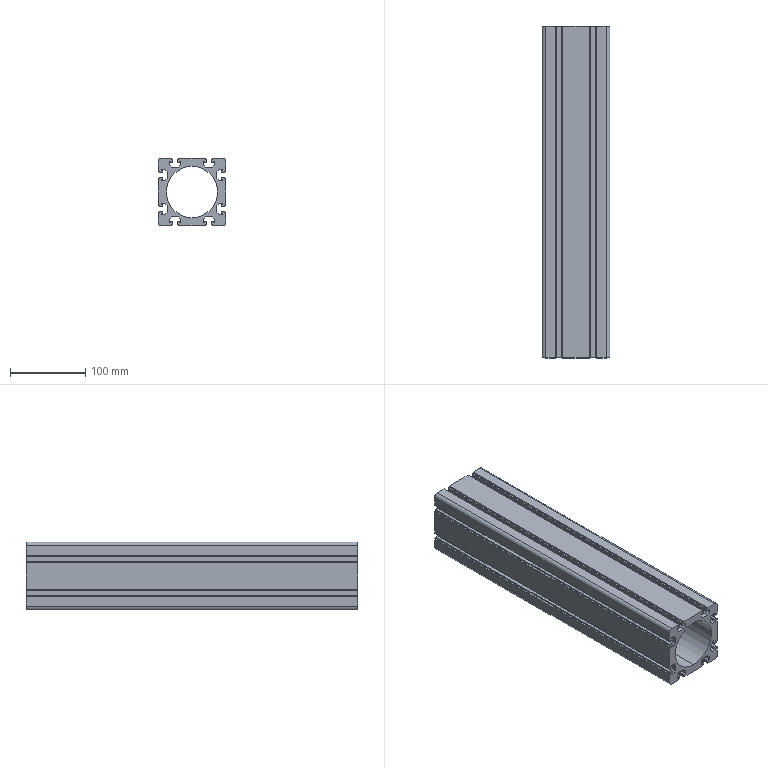Part | STEP file | leg01_5 | 1 solid | 156 faces | box 90 x 440 x 90 mm | volume 1490360 mm3 | plane 150 | cylinder 6 | commonest cylinder face diameters 10 x4 67.981 x2